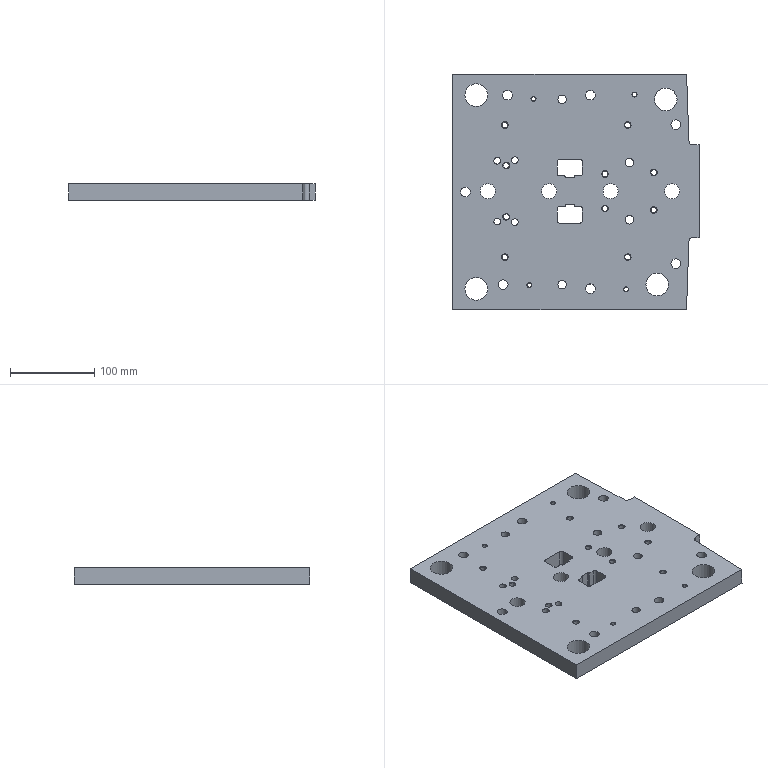Part | NX | features LB-10 2 | 1 solid | 101 faces | box 293 x 280 x 20 mm | volume 1469792 mm3 | cylinder 61 | plane 26 | cone 14 | commonest cylinder face diameters 6.8 x10 8 x10 1 x8 6 x8 11.5 x7 18.003 x4